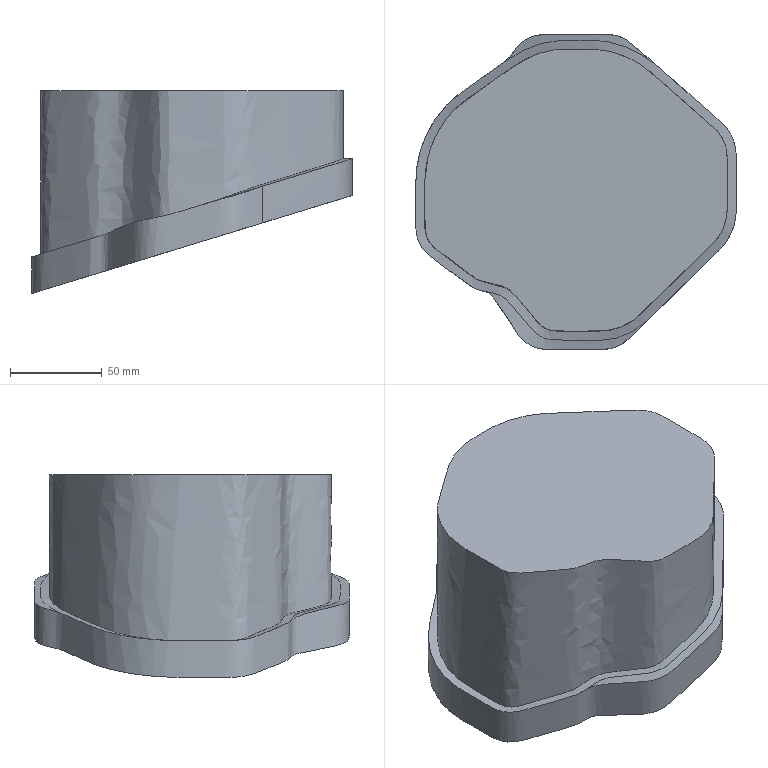Part | NX | features solid 2 | 1 solid | 25 faces | box 175.093 x 171.907 x 110.757 mm | volume 1156935 mm3 | spline 13 | plane 7 | cylinder 5 | commonest cylinder face diameters 30 x3 25 x2